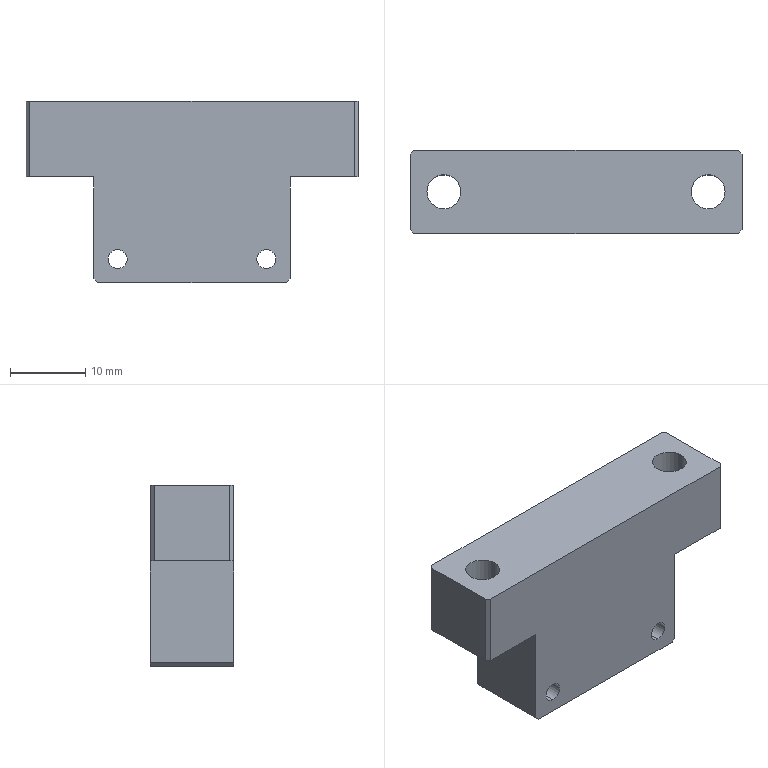Part | SolidWorks | features Chamfer 2, HoleWzd 2, Extrusion 1, ICE 1 | 1 solid | 30 faces | box 44 x 11 x 24 mm | volume 8094 mm3 | plane 18 | cylinder 12 | commonest cylinder face diameters 2.5 x4 4.5 x4 8 x4
STEP:
#1=CARTESIAN_POINT('',(9.85,-5.5,1.85));
#2=VERTEX_POINT('',#1);
#3=CARTESIAN_POINT('',(9.85,-5.5,4.35));
#4=VERTEX_POINT('',#3);
#5=CARTESIAN_POINT('',(9.85,-5.5,3.1));
#6=DIRECTION('',(0.,1.,0.));
#7=DIRECTION('',(0.,0.,1.));
#8=AXIS2_PLACEMENT_3D('',#5,#6,#7);
#9=CIRCLE('',#8,1.25);
#10=EDGE_CURVE('',#2,#4,#9,.T.);
#11=ORIENTED_EDGE('',*,*,#10,.F.);
#12=CARTESIAN_POINT('',(9.85,5.5,1.85));
#13=VERTEX_POINT('',#12);
#14=CARTESIAN_POINT('',(9.85,5.5,1.85));
#15=DIRECTION('',(0.,1.,0.));
#16=VECTOR('',#15,1000.);
#17=LINE('',#14,#16);
#18=EDGE_CURVE('',#2,#13,#17,.T.);
#19=ORIENTED_EDGE('',*,*,#18,.T.);
#20=CARTESIAN_POINT('',(9.85,5.5,4.35));
#21=VERTEX_POINT('',#20);
#22=CARTESIAN_POINT('',(9.85,5.5,3.1));
#23=DIRECTION('',(0.,1.,0.));
#24=DIRECTION('',(0.,0.,1.));
#25=AXIS2_PLACEMENT_3D('',#22,#23,#24);
#26=CIRCLE('',#25,1.25);
#27=EDGE_CURVE('',#13,#21,#26,.T.);
#28=ORIENTED_EDGE('',*,*,#27,.T.);
#29=CARTESIAN_POINT('',(9.85,5.5,4.35));
#30=DIRECTION('',(0.,1.,0.));
#31=VECTOR('',#30,1000.);
#32=LINE('',#29,#31);
#33=EDGE_CURVE('',#4,#21,#32,.T.);
#34=ORIENTED_EDGE('',*,*,#33,.F.);
#35=EDGE_LOOP('',(#11,#19,#28,#34));
#36=FACE_OUTER_BOUND('',#35,.T.);
#37=CARTESIAN_POINT('',(9.85,5.5,3.1));
#38=DIRECTION('',(0.,1.,0.));
#39=DIRECTION('',(0.,0.,1.));
#40=AXIS2_PLACEMENT_3D('',#37,#38,#39);
#41=CYLINDRICAL_SURFACE('',#40,1.25);
#42=ADVANCED_FACE('',(#36),#41,.F.);
#43=CARTESIAN_POINT('',(-9.85,-5.5,1.85));
#44=VERTEX_POINT('',#43);
#45=CARTESIAN_POINT('',(-9.85,-5.5,4.35));
#46=VERTEX_POINT('',#45);
#47=CARTESIAN_POINT('',(-9.85,-5.5,3.1));
#48=DIRECTION('',(0.,1.,0.));
#49=DIRECTION('',(0.,0.,1.));
#50=AXIS2_PLACEMENT_3D('',#47,#48,#49);
#51=CIRCLE('',#50,1.25);
#52=EDGE_CURVE('',#44,#46,#51,.T.);
#53=ORIENTED_EDGE('',*,*,#52,.F.);
#54=CARTESIAN_POINT('',(-9.85,5.5,1.85));
#55=VERTEX_POINT('',#54);
#56=CARTESIAN_POINT('',(-9.85,5.5,1.85));
#57=DIRECTION('',(0.,1.,0.));
#58=VECTOR('',#57,1000.);
#59=LINE('',#56,#58);
#60=EDGE_CURVE('',#44,#55,#59,.T.);
#61=ORIENTED_EDGE('',*,*,#60,.T.);
#62=CARTESIAN_POINT('',(-9.85,5.5,4.35));
#63=VERTEX_POINT('',#62);
#64=CARTESIAN_POINT('',(-9.85,5.5,3.1));
#65=DIRECTION('',(0.,1.,0.));
#66=DIRECTION('',(0.,0.,1.));
#67=AXIS2_PLACEMENT_3D('',#64,#65,#66);
#68=CIRCLE('',#67,1.25);
#69=EDGE_CURVE('',#55,#63,#68,.T.);
#70=ORIENTED_EDGE('',*,*,#69,.T.);
#71=CARTESIAN_POINT('',(-9.85,5.5,4.35));
#72=DIRECTION('',(0.,1.,0.));
#73=VECTOR('',#72,1000.);
#74=LINE('',#71,#73);
#75=EDGE_CURVE('',#46,#63,#74,.T.);
#76=ORIENTED_EDGE('',*,*,#75,.F.);
#77=EDGE_LOOP('',(#53,#61,#70,#76));
#78=FACE_OUTER_BOUND('',#77,.T.);
#79=CARTESIAN_POINT('',(-9.85,5.5,3.1));
#80=DIRECTION('',(0.,1.,0.));
#81=DIRECTION('',(0.,0.,1.));
#82=AXIS2_PLACEMENT_3D('',#79,#80,#81);
#83=CYLINDRICAL_SURFACE('',#82,1.25);
#84=ADVANCED_FACE('',(#78),#83,.F.);
#85=CARTESIAN_POINT('',(21.5,0.,18.6));
#86=VERTEX_POINT('',#85);
#87=CARTESIAN_POINT('',(13.5,0.,18.6));
#88=VERTEX_POINT('',#87);
#89=CARTESIAN_POINT('',(17.5,0.,18.6));
#90=DIRECTION('',(0.,0.,-1.));
#91=DIRECTION('',(-1.,0.,0.));
#92=AXIS2_PLACEMENT_3D('',#89,#90,#91);
#93=CIRCLE('',#92,4.);
#94=EDGE_CURVE('',#86,#88,#93,.T.);
#95=ORIENTED_EDGE('',*,*,#94,.F.);
#96=CARTESIAN_POINT('',(21.5,0.,14.));
#97=VERTEX_POINT('',#96);
#98=CARTESIAN_POINT('',(21.5,0.,14.));
#99=DIRECTION('',(0.,0.,-1.));
#100=VECTOR('',#99,1000.);
#101=LINE('',#98,#100);
#102=EDGE_CURVE('',#86,#97,#101,.T.);
#103=ORIENTED_EDGE('',*,*,#102,.T.);
#104=CARTESIAN_POINT('',(13.5,0.,14.));
#105=VERTEX_POINT('',#104);
#106=CARTESIAN_POINT('',(17.5,0.,14.));
#107=DIRECTION('',(0.,0.,-1.));
#108=DIRECTION('',(-1.,0.,0.));
#109=AXIS2_PLACEMENT_3D('',#106,#107,#108);
#110=CIRCLE('',#109,4.);
#111=EDGE_CURVE('',#97,#105,#110,.T.);
#112=ORIENTED_EDGE('',*,*,#111,.T.);
#113=CARTESIAN_POINT('',(13.5,0.,14.));
#114=DIRECTION('',(0.,0.,-1.));
#115=VECTOR('',#114,1000.);
#116=LINE('',#113,#115);
#117=EDGE_CURVE('',#88,#105,#116,.T.);
#118=ORIENTED_EDGE('',*,*,#117,.F.);
#119=EDGE_LOOP('',(#95,#103,#112,#118));
#120=FACE_OUTER_BOUND('',#119,.T.);
#121=CARTESIAN_POINT('',(17.5,0.,14.));
#122=DIRECTION('',(0.,0.,-1.));
#123=DIRECTION('',(-1.,0.,0.));
#124=AXIS2_PLACEMENT_3D('',#121,#122,#123);
#125=CYLINDRICAL_SURFACE('',#124,4.);
#126=ADVANCED_FACE('',(#120),#125,.F.);
#127=CARTESIAN_POINT('',(19.75,0.,24.));
#128=VERTEX_POINT('',#127);
#129=CARTESIAN_POINT('',(15.25,0.,24.));
#130=VERTEX_POINT('',#129);
#131=CARTESIAN_POINT('',(17.5,0.,24.));
#132=DIRECTION('',(0.,0.,-1.));
#133=DIRECTION('',(-1.,0.,0.));
#134=AXIS2_PLACEMENT_3D('',#131,#132,#133);
#135=CIRCLE('',#134,2.25);
#136=EDGE_CURVE('',#128,#130,#135,.T.);
#137=ORIENTED_EDGE('',*,*,#136,.F.);
#138=CARTESIAN_POINT('',(19.75,0.,18.6));
#139=VERTEX_POINT('',#138);
#140=CARTESIAN_POINT('',(19.75,0.,14.));
#141=DIRECTION('',(0.,0.,-1.));
#142=VECTOR('',#141,1000.);
#143=LINE('',#140,#142);
#144=EDGE_CURVE('',#128,#139,#143,.T.);
#145=ORIENTED_EDGE('',*,*,#144,.T.);
#146=CARTESIAN_POINT('',(15.25,0.,18.6));
#147=VERTEX_POINT('',#146);
#148=CARTESIAN_POINT('',(17.5,0.,18.6));
#149=DIRECTION('',(0.,0.,-1.));
#150=DIRECTION('',(-1.,0.,0.));
#151=AXIS2_PLACEMENT_3D('',#148,#149,#150);
#152=CIRCLE('',#151,2.25);
#153=EDGE_CURVE('',#139,#147,#152,.T.);
#154=ORIENTED_EDGE('',*,*,#153,.T.);
#155=CARTESIAN_POINT('',(15.25,0.,14.));
#156=DIRECTION('',(0.,0.,-1.));
#157=VECTOR('',#156,1000.);
#158=LINE('',#155,#157);
#159=EDGE_CURVE('',#130,#147,#158,.T.);
#160=ORIENTED_EDGE('',*,*,#159,.F.);
#161=EDGE_LOOP('',(#137,#145,#154,#160));
#162=FACE_OUTER_BOUND('',#161,.T.);
#163=CARTESIAN_POINT('',(17.5,0.,14.));
#164=DIRECTION('',(0.,0.,-1.));
#165=DIRECTION('',(-1.,0.,0.));
#166=AXIS2_PLACEMENT_3D('',#163,#164,#165);
#167=CYLINDRICAL_SURFACE('',#166,2.25);
#168=ADVANCED_FACE('',(#162),#167,.F.);
#169=CARTESIAN_POINT('',(-13.5,0.,18.6));
#170=VERTEX_POINT('',#169);
#171=CARTESIAN_POINT('',(-21.5,0.,18.6));
#172=VERTEX_POINT('',#171);
#173=CARTESIAN_POINT('',(-17.5,0.,18.6));
#174=DIRECTION('',(0.,0.,-1.));
#175=DIRECTION('',(-1.,0.,0.));
#176=AXIS2_PLACEMENT_3D('',#173,#174,#175);
#177=CIRCLE('',#176,4.);
#178=EDGE_CURVE('',#170,#172,#177,.T.);
#179=ORIENTED_EDGE('',*,*,#178,.F.);
#180=CARTESIAN_POINT('',(-13.5,0.,14.));
#181=VERTEX_POINT('',#180);
#182=CARTESIAN_POINT('',(-13.5,0.,14.));
#183=DIRECTION('',(0.,0.,-1.));
#184=VECTOR('',#183,1000.);
#185=LINE('',#182,#184);
#186=EDGE_CURVE('',#170,#181,#185,.T.);
#187=ORIENTED_EDGE('',*,*,#186,.T.);
#188=CARTESIAN_POINT('',(-21.5,0.,14.));
#189=VERTEX_POINT('',#188);
#190=CARTESIAN_POINT('',(-17.5,0.,14.));
#191=DIRECTION('',(0.,0.,-1.));
#192=DIRECTION('',(-1.,0.,0.));
#193=AXIS2_PLACEMENT_3D('',#190,#191,#192);
#194=CIRCLE('',#193,4.);
#195=EDGE_CURVE('',#181,#189,#194,.T.);
#196=ORIENTED_EDGE('',*,*,#195,.T.);
#197=CARTESIAN_POINT('',(-21.5,0.,14.));
#198=DIRECTION('',(0.,0.,-1.));
#199=VECTOR('',#198,1000.);
#200=LINE('',#197,#199);
#201=EDGE_CURVE('',#172,#189,#200,.T.);
#202=ORIENTED_EDGE('',*,*,#201,.F.);
#203=EDGE_LOOP('',(#179,#187,#196,#202));
#204=FACE_OUTER_BOUND('',#203,.T.);
#205=CARTESIAN_POINT('',(-17.5,0.,14.));
#206=DIRECTION('',(0.,0.,-1.));
#207=DIRECTION('',(-1.,0.,0.));
#208=AXIS2_PLACEMENT_3D('',#205,#206,#207);
#209=CYLINDRICAL_SURFACE('',#208,4.);
#210=ADVANCED_FACE('',(#204),#209,.F.);
#211=CARTESIAN_POINT('',(-15.25,0.,24.));
#212=VERTEX_POINT('',#211);
#213=CARTESIAN_POINT('',(-19.75,0.,24.));
#214=VERTEX_POINT('',#213);
#215=CARTESIAN_POINT('',(-17.5,0.,24.));
#216=DIRECTION('',(0.,0.,-1.));
#217=DIRECTION('',(-1.,0.,0.));
#218=AXIS2_PLACEMENT_3D('',#215,#216,#217);
#219=CIRCLE('',#218,2.25);
#220=EDGE_CURVE('',#212,#214,#219,.T.);
#221=ORIENTED_EDGE('',*,*,#220,.F.);
#222=CARTESIAN_POINT('',(-15.25,0.,18.6));
#223=VERTEX_POINT('',#222);
#224=CARTESIAN_POINT('',(-15.25,0.,14.));
#225=DIRECTION('',(0.,0.,-1.));
#226=VECTOR('',#225,1000.);
#227=LINE('',#224,#226);
#228=EDGE_CURVE('',#212,#223,#227,.T.);
#229=ORIENTED_EDGE('',*,*,#228,.T.);
#230=CARTESIAN_POINT('',(-19.75,0.,18.6));
#231=VERTEX_POINT('',#230);
#232=CARTESIAN_POINT('',(-17.5,0.,18.6));
#233=DIRECTION('',(0.,0.,-1.));
#234=DIRECTION('',(-1.,0.,0.));
#235=AXIS2_PLACEMENT_3D('',#232,#233,#234);
#236=CIRCLE('',#235,2.25);
#237=EDGE_CURVE('',#223,#231,#236,.T.);
#238=ORIENTED_EDGE('',*,*,#237,.T.);
#239=CARTESIAN_POINT('',(-19.75,0.,14.));
#240=DIRECTION('',(0.,0.,-1.));
#241=VECTOR('',#240,1000.);
#242=LINE('',#239,#241);
#243=EDGE_CURVE('',#214,#231,#242,.T.);
#244=ORIENTED_EDGE('',*,*,#243,.F.);
#245=EDGE_LOOP('',(#221,#229,#238,#244));
#246=FACE_OUTER_BOUND('',#245,.T.);
#247=CARTESIAN_POINT('',(-17.5,0.,14.));
#248=DIRECTION('',(0.,0.,-1.));
#249=DIRECTION('',(-1.,0.,0.));
#250=AXIS2_PLACEMENT_3D('',#247,#248,#249);
#251=CYLINDRICAL_SURFACE('',#250,2.25);
#252=ADVANCED_FACE('',(#246),#251,.F.);
#253=CARTESIAN_POINT('',(13.,5.5,14.));
#254=VERTEX_POINT('',#253);
#255=CARTESIAN_POINT('',(21.5,5.5,14.));
#256=VERTEX_POINT('',#255);
#257=CARTESIAN_POINT('',(22.,5.5,14.));
#258=DIRECTION('',(1.,0.,0.));
#259=VECTOR('',#258,1000.);
#260=LINE('',#257,#259);
#261=EDGE_CURVE('',#254,#256,#260,.T.);
#262=ORIENTED_EDGE('',*,*,#261,.T.);
#263=CARTESIAN_POINT('',(22.,5.,14.));
#264=VERTEX_POINT('',#263);
#265=CARTESIAN_POINT('',(21.5,5.5,14.));
#266=DIRECTION('',(0.7071,-0.7071,0.));
#267=VECTOR('',#266,1000.);
#268=LINE('',#265,#267);
#269=EDGE_CURVE('',#256,#264,#268,.T.);
#270=ORIENTED_EDGE('',*,*,#269,.T.);
#271=CARTESIAN_POINT('',(22.,-5.,14.));
#272=VERTEX_POINT('',#271);
#273=CARTESIAN_POINT('',(22.,-5.5,14.));
#274=DIRECTION('',(0.,1.,0.));
#275=VECTOR('',#274,1000.);
#276=LINE('',#273,#275);
#277=EDGE_CURVE('',#272,#264,#276,.T.);
#278=ORIENTED_EDGE('',*,*,#277,.F.);
#279=CARTESIAN_POINT('',(21.5,-5.5,14.));
#280=VERTEX_POINT('',#279);
#281=CARTESIAN_POINT('',(22.,-5.,14.));
#282=DIRECTION('',(-0.7071,-0.7071,0.));
#283=VECTOR('',#282,1000.);
#284=LINE('',#281,#283);
#285=EDGE_CURVE('',#272,#280,#284,.T.);
#286=ORIENTED_EDGE('',*,*,#285,.T.);
#287=CARTESIAN_POINT('',(13.,-5.5,14.));
#288=VERTEX_POINT('',#287);
#289=CARTESIAN_POINT('',(22.,-5.5,14.));
#290=DIRECTION('',(1.,0.,0.));
#291=VECTOR('',#290,1000.);
#292=LINE('',#289,#291);
#293=EDGE_CURVE('',#288,#280,#292,.T.);
#294=ORIENTED_EDGE('',*,*,#293,.F.);
#295=CARTESIAN_POINT('',(13.,-5.5,14.));
#296=DIRECTION('',(0.,1.,0.));
#297=VECTOR('',#296,1000.);
#298=LINE('',#295,#297);
#299=EDGE_CURVE('',#288,#254,#298,.T.);
#300=ORIENTED_EDGE('',*,*,#299,.T.);
#301=EDGE_LOOP('',(#262,#270,#278,#286,#294,#300));
#302=FACE_OUTER_BOUND('',#301,.T.);
#303=CARTESIAN_POINT('',(17.5,0.,14.));
#304=DIRECTION('',(0.,0.,-1.));
#305=DIRECTION('',(-1.,0.,0.));
#306=AXIS2_PLACEMENT_3D('',#303,#304,#305);
#307=CIRCLE('',#306,4.);
#308=EDGE_CURVE('',#105,#97,#307,.T.);
#309=ORIENTED_EDGE('',*,*,#308,.F.);
#310=ORIENTED_EDGE('',*,*,#111,.F.);
#311=EDGE_LOOP('',(#309,#310));
#312=FACE_BOUND('',#311,.T.);
#313=CARTESIAN_POINT('',(22.,-5.5,14.));
#314=DIRECTION('',(0.,0.,1.));
#315=DIRECTION('',(1.,0.,0.));
#316=AXIS2_PLACEMENT_3D('',#313,#314,#315);
#317=PLANE('',#316);
#318=ADVANCED_FACE('',(#302,#312),#317,.F.);
#319=ORIENTED_EDGE('',*,*,#277,.T.);
#320=CARTESIAN_POINT('',(22.,5.,24.));
#321=VERTEX_POINT('',#320);
#322=CARTESIAN_POINT('',(22.,5.,24.));
#323=DIRECTION('',(0.,0.,1.));
#324=VECTOR('',#323,1000.);
#325=LINE('',#322,#324);
#326=EDGE_CURVE('',#264,#321,#325,.T.);
#327=ORIENTED_EDGE('',*,*,#326,.T.);
#328=CARTESIAN_POINT('',(22.,-5.,24.));
#329=VERTEX_POINT('',#328);
#330=CARTESIAN_POINT('',(22.,5.5,24.));
#331=DIRECTION('',(0.,1.,0.));
#332=VECTOR('',#331,1000.);
#333=LINE('',#330,#332);
#334=EDGE_CURVE('',#329,#321,#333,.T.);
#335=ORIENTED_EDGE('',*,*,#334,.F.);
#336=CARTESIAN_POINT('',(22.,-5.,24.));
#337=DIRECTION('',(0.,0.,-1.));
#338=VECTOR('',#337,1000.);
#339=LINE('',#336,#338);
#340=EDGE_CURVE('',#329,#272,#339,.T.);
#341=ORIENTED_EDGE('',*,*,#340,.T.);
#342=EDGE_LOOP('',(#319,#327,#335,#341));
#343=FACE_OUTER_BOUND('',#342,.T.);
#344=CARTESIAN_POINT('',(22.,5.5,24.));
#345=DIRECTION('',(-1.,0.,0.));
#346=DIRECTION('',(0.,0.,1.));
#347=AXIS2_PLACEMENT_3D('',#344,#345,#346);
#348=PLANE('',#347);
#349=ADVANCED_FACE('',(#343),#348,.F.);
#350=CARTESIAN_POINT('',(9.85,5.5,3.1));
#351=DIRECTION('',(0.,1.,0.));
#352=DIRECTION('',(0.,0.,1.));
#353=AXIS2_PLACEMENT_3D('',#350,#351,#352);
#354=CIRCLE('',#353,1.25);
#355=EDGE_CURVE('',#21,#13,#354,.T.);
#356=ORIENTED_EDGE('',*,*,#355,.F.);
#357=ORIENTED_EDGE('',*,*,#27,.F.);
#358=EDGE_LOOP('',(#356,#357));
#359=FACE_BOUND('',#358,.T.);
#360=CARTESIAN_POINT('',(-9.85,5.5,3.1));
#361=DIRECTION('',(0.,1.,0.));
#362=DIRECTION('',(0.,0.,1.));
#363=AXIS2_PLACEMENT_3D('',#360,#361,#362);
#364=CIRCLE('',#363,1.25);
#365=EDGE_CURVE('',#63,#55,#364,.T.);
#366=ORIENTED_EDGE('',*,*,#365,.F.);
#367=ORIENTED_EDGE('',*,*,#69,.F.);
#368=EDGE_LOOP('',(#366,#367));
#369=FACE_BOUND('',#368,.T.);
#370=CARTESIAN_POINT('',(13.,5.5,0.5));
#371=VERTEX_POINT('',#370);
#372=CARTESIAN_POINT('',(13.,5.5,14.));
#373=DIRECTION('',(0.,0.,1.));
#374=VECTOR('',#373,1000.);
#375=LINE('',#372,#374);
#376=EDGE_CURVE('',#371,#254,#375,.T.);
#377=ORIENTED_EDGE('',*,*,#376,.F.);
#378=CARTESIAN_POINT('',(12.5,5.5,0.));
#379=VERTEX_POINT('',#378);
#380=CARTESIAN_POINT('',(13.,5.5,0.5));
#381=DIRECTION('',(-0.7071,0.,-0.7071));
#382=VECTOR('',#381,1000.);
#383=LINE('',#380,#382);
#384=EDGE_CURVE('',#371,#379,#383,.T.);
#385=ORIENTED_EDGE('',*,*,#384,.T.);
#386=CARTESIAN_POINT('',(-12.5,5.5,0.));
#387=VERTEX_POINT('',#386);
#388=CARTESIAN_POINT('',(-22.,5.5,0.));
#389=DIRECTION('',(-1.,0.,0.));
#390=VECTOR('',#389,1000.);
#391=LINE('',#388,#390);
#392=EDGE_CURVE('',#379,#387,#391,.T.);
#393=ORIENTED_EDGE('',*,*,#392,.T.);
#394=CARTESIAN_POINT('',(-13.,5.5,0.5));
#395=VERTEX_POINT('',#394);
#396=CARTESIAN_POINT('',(-12.5,5.5,0.));
#397=DIRECTION('',(-0.7071,0.,0.7071));
#398=VECTOR('',#397,1000.);
#399=LINE('',#396,#398);
#400=EDGE_CURVE('',#387,#395,#399,.T.);
#401=ORIENTED_EDGE('',*,*,#400,.T.);
#402=CARTESIAN_POINT('',(-13.,5.5,14.));
#403=VERTEX_POINT('',#402);
#404=CARTESIAN_POINT('',(-13.,5.5,14.));
#405=DIRECTION('',(0.,0.,-1.));
#406=VECTOR('',#405,1000.);
#407=LINE('',#404,#406);
#408=EDGE_CURVE('',#403,#395,#407,.T.);
#409=ORIENTED_EDGE('',*,*,#408,.F.);
#410=CARTESIAN_POINT('',(-21.5,5.5,14.));
#411=VERTEX_POINT('',#410);
#412=CARTESIAN_POINT('',(-22.,5.5,14.));
#413=DIRECTION('',(1.,0.,0.));
#414=VECTOR('',#413,1000.);
#415=LINE('',#412,#414);
#416=EDGE_CURVE('',#411,#403,#415,.T.);
#417=ORIENTED_EDGE('',*,*,#416,.F.);
#418=CARTESIAN_POINT('',(-21.5,5.5,24.));
#419=VERTEX_POINT('',#418);
#420=CARTESIAN_POINT('',(-21.5,5.5,24.));
#421=DIRECTION('',(0.,0.,1.));
#422=VECTOR('',#421,1000.);
#423=LINE('',#420,#422);
#424=EDGE_CURVE('',#411,#419,#423,.T.);
#425=ORIENTED_EDGE('',*,*,#424,.T.);
#426=CARTESIAN_POINT('',(21.5,5.5,24.));
#427=VERTEX_POINT('',#426);
#428=CARTESIAN_POINT('',(-22.,5.5,24.));
#429=DIRECTION('',(-1.,0.,0.));
#430=VECTOR('',#429,1000.);
#431=LINE('',#428,#430);
#432=EDGE_CURVE('',#427,#419,#431,.T.);
#433=ORIENTED_EDGE('',*,*,#432,.F.);
#434=CARTESIAN_POINT('',(21.5,5.5,24.));
#435=DIRECTION('',(0.,0.,-1.));
#436=VECTOR('',#435,1000.);
#437=LINE('',#434,#436);
#438=EDGE_CURVE('',#427,#256,#437,.T.);
#439=ORIENTED_EDGE('',*,*,#438,.T.);
#440=ORIENTED_EDGE('',*,*,#261,.F.);
#441=EDGE_LOOP('',(#377,#385,#393,#401,#409,#417,#425,#433,#439,#440));
#442=FACE_OUTER_BOUND('',#441,.T.);
#443=CARTESIAN_POINT('',(-22.,5.5,24.));
#444=DIRECTION('',(0.,-1.,0.));
#445=DIRECTION('',(0.,0.,-1.));
#446=AXIS2_PLACEMENT_3D('',#443,#444,#445);
#447=PLANE('',#446);
#448=ADVANCED_FACE('',(#359,#369,#442),#447,.F.);
#449=CARTESIAN_POINT('',(-22.,5.,24.));
#450=VERTEX_POINT('',#449);
#451=CARTESIAN_POINT('',(-22.,-5.,24.));
#452=VERTEX_POINT('',#451);
#453=CARTESIAN_POINT('',(-22.,5.5,24.));
#454=DIRECTION('',(0.,-1.,0.));
#455=VECTOR('',#454,1000.);
#456=LINE('',#453,#455);
#457=EDGE_CURVE('',#450,#452,#456,.T.);
#458=ORIENTED_EDGE('',*,*,#457,.F.);
#459=CARTESIAN_POINT('',(-22.,5.,14.));
#460=VERTEX_POINT('',#459);
#461=CARTESIAN_POINT('',(-22.,5.,24.));
#462=DIRECTION('',(0.,0.,-1.));
#463=VECTOR('',#462,1000.);
#464=LINE('',#461,#463);
#465=EDGE_CURVE('',#450,#460,#464,.T.);
#466=ORIENTED_EDGE('',*,*,#465,.T.);
#467=CARTESIAN_POINT('',(-22.,-5.,14.));
#468=VERTEX_POINT('',#467);
#469=CARTESIAN_POINT('',(-22.,-5.5,14.));
#470=DIRECTION('',(0.,1.,0.));
#471=VECTOR('',#470,1000.);
#472=LINE('',#469,#471);
#473=EDGE_CURVE('',#468,#460,#472,.T.);
#474=ORIENTED_EDGE('',*,*,#473,.F.);
#475=CARTESIAN_POINT('',(-22.,-5.,24.));
#476=DIRECTION('',(0.,0.,1.));
#477=VECTOR('',#476,1000.);
#478=LINE('',#475,#477);
#479=EDGE_CURVE('',#468,#452,#478,.T.);
#480=ORIENTED_EDGE('',*,*,#479,.T.);
#481=EDGE_LOOP('',(#458,#466,#474,#480));
#482=FACE_OUTER_BOUND('',#481,.T.);
#483=CARTESIAN_POINT('',(-22.,5.5,24.));
#484=DIRECTION('',(1.,0.,0.));
#485=DIRECTION('',(0.,0.,-1.));
#486=AXIS2_PLACEMENT_3D('',#483,#484,#485);
#487=PLANE('',#486);
#488=ADVANCED_FACE('',(#482),#487,.F.);
#489=CARTESIAN_POINT('',(9.85,-5.5,3.1));
#490=DIRECTION('',(0.,1.,0.));
#491=DIRECTION('',(0.,0.,1.));
#492=AXIS2_PLACEMENT_3D('',#489,#490,#491);
#493=CIRCLE('',#492,1.25);
#494=EDGE_CURVE('',#4,#2,#493,.T.);
#495=ORIENTED_EDGE('',*,*,#494,.T.);
#496=ORIENTED_EDGE('',*,*,#10,.T.);
#497=EDGE_LOOP('',(#495,#496));
#498=FACE_BOUND('',#497,.T.);
#499=CARTESIAN_POINT('',(-9.85,-5.5,3.1));
#500=DIRECTION('',(0.,1.,0.));
#501=DIRECTION('',(0.,0.,1.));
#502=AXIS2_PLACEMENT_3D('',#499,#500,#501);
#503=CIRCLE('',#502,1.25);
#504=EDGE_CURVE('',#46,#44,#503,.T.);
#505=ORIENTED_EDGE('',*,*,#504,.T.);
#506=ORIENTED_EDGE('',*,*,#52,.T.);
#507=EDGE_LOOP('',(#505,#506));
#508=FACE_BOUND('',#507,.T.);
#509=CARTESIAN_POINT('',(-12.5,-5.5,0.));
#510=VERTEX_POINT('',#509);
#511=CARTESIAN_POINT('',(12.5,-5.5,0.));
#512=VERTEX_POINT('',#511);
#513=CARTESIAN_POINT('',(-22.,-5.5,0.));
#514=DIRECTION('',(1.,0.,0.));
#515=VECTOR('',#514,1000.);
#516=LINE('',#513,#515);
#517=EDGE_CURVE('',#510,#512,#516,.T.);
#518=ORIENTED_EDGE('',*,*,#517,.T.);
#519=CARTESIAN_POINT('',(13.,-5.5,0.5));
#520=VERTEX_POINT('',#519);
#521=CARTESIAN_POINT('',(13.,-5.5,0.5));
#522=DIRECTION('',(0.7071,0.,0.7071));
#523=VECTOR('',#522,1000.);
#524=LINE('',#521,#523);
#525=EDGE_CURVE('',#512,#520,#524,.T.);
#526=ORIENTED_EDGE('',*,*,#525,.T.);
#527=CARTESIAN_POINT('',(13.,-5.5,14.));
#528=DIRECTION('',(0.,0.,1.));
#529=VECTOR('',#528,1000.);
#530=LINE('',#527,#529);
#531=EDGE_CURVE('',#520,#288,#530,.T.);
#532=ORIENTED_EDGE('',*,*,#531,.T.);
#533=ORIENTED_EDGE('',*,*,#293,.T.);
#534=CARTESIAN_POINT('',(21.5,-5.5,24.));
#535=VERTEX_POINT('',#534);
#536=CARTESIAN_POINT('',(21.5,-5.5,24.));
#537=DIRECTION('',(0.,0.,1.));
#538=VECTOR('',#537,1000.);
#539=LINE('',#536,#538);
#540=EDGE_CURVE('',#280,#535,#539,.T.);
#541=ORIENTED_EDGE('',*,*,#540,.T.);
#542=CARTESIAN_POINT('',(-21.5,-5.5,24.));
#543=VERTEX_POINT('',#542);
#544=CARTESIAN_POINT('',(-22.,-5.5,24.));
#545=DIRECTION('',(1.,0.,0.));
#546=VECTOR('',#545,1000.);
#547=LINE('',#544,#546);
#548=EDGE_CURVE('',#543,#535,#547,.T.);
#549=ORIENTED_EDGE('',*,*,#548,.F.);
#550=CARTESIAN_POINT('',(-21.5,-5.5,14.));
#551=VERTEX_POINT('',#550);
#552=CARTESIAN_POINT('',(-21.5,-5.5,24.));
#553=DIRECTION('',(0.,0.,-1.));
#554=VECTOR('',#553,1000.);
#555=LINE('',#552,#554);
#556=EDGE_CURVE('',#543,#551,#555,.T.);
#557=ORIENTED_EDGE('',*,*,#556,.T.);
#558=CARTESIAN_POINT('',(-13.,-5.5,14.));
#559=VERTEX_POINT('',#558);
#560=CARTESIAN_POINT('',(-22.,-5.5,14.));
#561=DIRECTION('',(1.,0.,0.));
#562=VECTOR('',#561,1000.);
#563=LINE('',#560,#562);
#564=EDGE_CURVE('',#551,#559,#563,.T.);
#565=ORIENTED_EDGE('',*,*,#564,.T.);
#566=CARTESIAN_POINT('',(-13.,-5.5,0.5));
#567=VERTEX_POINT('',#566);
#568=CARTESIAN_POINT('',(-13.,-5.5,14.));
#569=DIRECTION('',(0.,0.,-1.));
#570=VECTOR('',#569,1000.);
#571=LINE('',#568,#570);
#572=EDGE_CURVE('',#559,#567,#571,.T.);
#573=ORIENTED_EDGE('',*,*,#572,.T.);
#574=CARTESIAN_POINT('',(-12.5,-5.5,0.));
#575=DIRECTION('',(0.7071,0.,-0.7071));
#576=VECTOR('',#575,1000.);
#577=LINE('',#574,#576);
#578=EDGE_CURVE('',#567,#510,#577,.T.);
#579=ORIENTED_EDGE('',*,*,#578,.T.);
#580=EDGE_LOOP('',(#518,#526,#532,#533,#541,#549,#557,#565,#573,#579));
#581=FACE_OUTER_BOUND('',#580,.T.);
#582=CARTESIAN_POINT('',(-22.,-5.5,24.));
#583=DIRECTION('',(0.,1.,0.));
#584=DIRECTION('',(0.,0.,1.));
#585=AXIS2_PLACEMENT_3D('',#582,#583,#584);
#586=PLANE('',#585);
#587=ADVANCED_FACE('',(#498,#508,#581),#586,.F.);
#588=CARTESIAN_POINT('',(17.5,0.,24.));
#589=DIRECTION('',(0.,0.,-1.));
#590=DIRECTION('',(-1.,0.,0.));
#591=AXIS2_PLACEMENT_3D('',#588,#589,#590);
#592=CIRCLE('',#591,2.25);
#593=EDGE_CURVE('',#130,#128,#592,.T.);
#594=ORIENTED_EDGE('',*,*,#593,.T.);
#595=ORIENTED_EDGE('',*,*,#136,.T.);
#596=EDGE_LOOP('',(#594,#595));
#597=FACE_BOUND('',#596,.T.);
#598=CARTESIAN_POINT('',(-17.5,0.,24.));
#599=DIRECTION('',(0.,0.,-1.));
#600=DIRECTION('',(-1.,0.,0.));
#601=AXIS2_PLACEMENT_3D('',#598,#599,#600);
#602=CIRCLE('',#601,2.25);
#603=EDGE_CURVE('',#214,#212,#602,.T.);
#604=ORIENTED_EDGE('',*,*,#603,.T.);
#605=ORIENTED_EDGE('',*,*,#220,.T.);
#606=EDGE_LOOP('',(#604,#605));
#607=FACE_BOUND('',#606,.T.);
#608=ORIENTED_EDGE('',*,*,#334,.T.);
#609=CARTESIAN_POINT('',(13.5,13.5,24.));
#610=DIRECTION('',(-0.7071,0.7071,0.));
#611=VECTOR('',#610,1000.);
#612=LINE('',#609,#611);
#613=EDGE_CURVE('',#321,#427,#612,.T.);
#614=ORIENTED_EDGE('',*,*,#613,.T.);
#615=ORIENTED_EDGE('',*,*,#432,.T.);
#616=CARTESIAN_POINT('',(-13.5,13.5,24.));
#617=DIRECTION('',(-0.7071,-0.7071,0.));
#618=VECTOR('',#617,1000.);
#619=LINE('',#616,#618);
#620=EDGE_CURVE('',#419,#450,#619,.T.);
#621=ORIENTED_EDGE('',*,*,#620,.T.);
#622=ORIENTED_EDGE('',*,*,#457,.T.);
#623=CARTESIAN_POINT('',(-13.5,-13.5,24.));
#624=DIRECTION('',(0.7071,-0.7071,0.));
#625=VECTOR('',#624,1000.);
#626=LINE('',#623,#625);
#627=EDGE_CURVE('',#452,#543,#626,.T.);
#628=ORIENTED_EDGE('',*,*,#627,.T.);
#629=ORIENTED_EDGE('',*,*,#548,.T.);
#630=CARTESIAN_POINT('',(13.5,-13.5,24.));
#631=DIRECTION('',(0.7071,0.7071,0.));
#632=VECTOR('',#631,1000.);
#633=LINE('',#630,#632);
#634=EDGE_CURVE('',#535,#329,#633,.T.);
#635=ORIENTED_EDGE('',*,*,#634,.T.);
#636=EDGE_LOOP('',(#608,#614,#615,#621,#622,#628,#629,#635));
#637=FACE_OUTER_BOUND('',#636,.T.);
#638=CARTESIAN_POINT('',(0.,0.,24.));
#639=DIRECTION('',(0.,0.,1.));
#640=DIRECTION('',(1.,0.,0.));
#641=AXIS2_PLACEMENT_3D('',#638,#639,#640);
#642=PLANE('',#641);
#643=ADVANCED_FACE('',(#597,#607,#637),#642,.T.);
#644=ORIENTED_EDGE('',*,*,#392,.F.);
#645=CARTESIAN_POINT('',(12.5,0.,0.));
#646=DIRECTION('',(0.,-1.,0.));
#647=VECTOR('',#646,1000.);
#648=LINE('',#645,#647);
#649=EDGE_CURVE('',#379,#512,#648,.T.);
#650=ORIENTED_EDGE('',*,*,#649,.T.);
#651=ORIENTED_EDGE('',*,*,#517,.F.);
#652=CARTESIAN_POINT('',(-12.5,0.,0.));
#653=DIRECTION('',(0.,1.,0.));
#654=VECTOR('',#653,1000.);
#655=LINE('',#652,#654);
#656=EDGE_CURVE('',#510,#387,#655,.T.);
#657=ORIENTED_EDGE('',*,*,#656,.T.);
#658=EDGE_LOOP('',(#644,#650,#651,#657));
#659=FACE_OUTER_BOUND('',#658,.T.);
#660=CARTESIAN_POINT('',(0.,0.,0.));
#661=DIRECTION('',(0.,0.,1.));
#662=DIRECTION('',(1.,0.,0.));
#663=AXIS2_PLACEMENT_3D('',#660,#661,#662);
#664=PLANE('',#663);
#665=ADVANCED_FACE('',(#659),#664,.F.);
#666=ORIENTED_EDGE('',*,*,#531,.F.);
#667=CARTESIAN_POINT('',(13.,-5.5,0.5));
#668=DIRECTION('',(0.,1.,0.));
#669=VECTOR('',#668,1000.);
#670=LINE('',#667,#669);
#671=EDGE_CURVE('',#520,#371,#670,.T.);
#672=ORIENTED_EDGE('',*,*,#671,.T.);
#673=ORIENTED_EDGE('',*,*,#376,.T.);
#674=ORIENTED_EDGE('',*,*,#299,.F.);
#675=EDGE_LOOP('',(#666,#672,#673,#674));
#676=FACE_OUTER_BOUND('',#675,.T.);
#677=CARTESIAN_POINT('',(13.,-5.5,14.));
#678=DIRECTION('',(-1.,0.,0.));
#679=DIRECTION('',(0.,0.,1.));
#680=AXIS2_PLACEMENT_3D('',#677,#678,#679);
#681=PLANE('',#680);
#682=ADVANCED_FACE('',(#676),#681,.F.);
#683=ORIENTED_EDGE('',*,*,#408,.T.);
#684=CARTESIAN_POINT('',(-13.,-5.5,0.5));
#685=DIRECTION('',(0.,-1.,0.));
#686=VECTOR('',#685,1000.);
#687=LINE('',#684,#686);
#688=EDGE_CURVE('',#395,#567,#687,.T.);
#689=ORIENTED_EDGE('',*,*,#688,.T.);
#690=ORIENTED_EDGE('',*,*,#572,.F.);
#691=CARTESIAN_POINT('',(-13.,-5.5,14.));
#692=DIRECTION('',(0.,1.,0.));
#693=VECTOR('',#692,1000.);
#694=LINE('',#691,#693);
#695=EDGE_CURVE('',#559,#403,#694,.T.);
#696=ORIENTED_EDGE('',*,*,#695,.T.);
#697=EDGE_LOOP('',(#683,#689,#690,#696));
#698=FACE_OUTER_BOUND('',#697,.T.);
#699=CARTESIAN_POINT('',(-13.,-5.5,14.));
#700=DIRECTION('',(1.,0.,0.));
#701=DIRECTION('',(0.,0.,-1.));
#702=AXIS2_PLACEMENT_3D('',#699,#700,#701);
#703=PLANE('',#702);
#704=ADVANCED_FACE('',(#698),#703,.F.);
#705=CARTESIAN_POINT('',(-17.5,0.,14.));
#706=DIRECTION('',(0.,0.,-1.));
#707=DIRECTION('',(-1.,0.,0.));
#708=AXIS2_PLACEMENT_3D('',#705,#706,#707);
#709=CIRCLE('',#708,4.);
#710=EDGE_CURVE('',#189,#181,#709,.T.);
#711=ORIENTED_EDGE('',*,*,#710,.F.);
#712=ORIENTED_EDGE('',*,*,#195,.F.);
#713=EDGE_LOOP('',(#711,#712));
#714=FACE_BOUND('',#713,.T.);
#715=ORIENTED_EDGE('',*,*,#473,.T.);
#716=CARTESIAN_POINT('',(-22.,5.,14.));
#717=DIRECTION('',(0.7071,0.7071,0.));
#718=VECTOR('',#717,1000.);
#719=LINE('',#716,#718);
#720=EDGE_CURVE('',#460,#411,#719,.T.);
#721=ORIENTED_EDGE('',*,*,#720,.T.);
#722=ORIENTED_EDGE('',*,*,#416,.T.);
#723=ORIENTED_EDGE('',*,*,#695,.F.);
#724=ORIENTED_EDGE('',*,*,#564,.F.);
#725=CARTESIAN_POINT('',(-21.5,-5.5,14.));
#726=DIRECTION('',(-0.7071,0.7071,0.));
#727=VECTOR('',#726,1000.);
#728=LINE('',#725,#727);
#729=EDGE_CURVE('',#551,#468,#728,.T.);
#730=ORIENTED_EDGE('',*,*,#729,.T.);
#731=EDGE_LOOP('',(#715,#721,#722,#723,#724,#730));
#732=FACE_OUTER_BOUND('',#731,.T.);
#733=CARTESIAN_POINT('',(-22.,-5.5,14.));
#734=DIRECTION('',(0.,0.,1.));
#735=DIRECTION('',(1.,0.,0.));
#736=AXIS2_PLACEMENT_3D('',#733,#734,#735);
#737=PLANE('',#736);
#738=ADVANCED_FACE('',(#714,#732),#737,.F.);
#739=ORIENTED_EDGE('',*,*,#228,.F.);
#740=ORIENTED_EDGE('',*,*,#603,.F.);
#741=ORIENTED_EDGE('',*,*,#243,.T.);
#742=CARTESIAN_POINT('',(-17.5,0.,18.6));
#743=DIRECTION('',(0.,0.,-1.));
#744=DIRECTION('',(-1.,0.,0.));
#745=AXIS2_PLACEMENT_3D('',#742,#743,#744);
#746=CIRCLE('',#745,2.25);
#747=EDGE_CURVE('',#231,#223,#746,.T.);
#748=ORIENTED_EDGE('',*,*,#747,.T.);
#749=EDGE_LOOP('',(#739,#740,#741,#748));
#750=FACE_OUTER_BOUND('',#749,.T.);
#751=CARTESIAN_POINT('',(-17.5,0.,14.));
#752=DIRECTION('',(0.,0.,-1.));
#753=DIRECTION('',(-1.,0.,0.));
#754=AXIS2_PLACEMENT_3D('',#751,#752,#753);
#755=CYLINDRICAL_SURFACE('',#754,2.25);
#756=ADVANCED_FACE('',(#750),#755,.F.);
#757=ORIENTED_EDGE('',*,*,#747,.F.);
#758=ORIENTED_EDGE('',*,*,#237,.F.);
#759=EDGE_LOOP('',(#757,#758));
#760=FACE_BOUND('',#759,.T.);
#761=CARTESIAN_POINT('',(-17.5,0.,18.6));
#762=DIRECTION('',(0.,0.,-1.));
#763=DIRECTION('',(-1.,0.,0.));
#764=AXIS2_PLACEMENT_3D('',#761,#762,#763);
#765=CIRCLE('',#764,4.);
#766=EDGE_CURVE('',#172,#170,#765,.T.);
#767=ORIENTED_EDGE('',*,*,#766,.T.);
#768=ORIENTED_EDGE('',*,*,#178,.T.);
#769=EDGE_LOOP('',(#767,#768));
#770=FACE_OUTER_BOUND('',#769,.T.);
#771=CARTESIAN_POINT('',(-15.25,0.,18.6));
#772=DIRECTION('',(0.,0.,1.));
#773=DIRECTION('',(1.,0.,0.));
#774=AXIS2_PLACEMENT_3D('',#771,#772,#773);
#775=PLANE('',#774);
#776=ADVANCED_FACE('',(#760,#770),#775,.F.);
#777=ORIENTED_EDGE('',*,*,#186,.F.);
#778=ORIENTED_EDGE('',*,*,#766,.F.);
#779=ORIENTED_EDGE('',*,*,#201,.T.);
#780=ORIENTED_EDGE('',*,*,#710,.T.);
#781=EDGE_LOOP('',(#777,#778,#779,#780));
#782=FACE_OUTER_BOUND('',#781,.T.);
#783=CARTESIAN_POINT('',(-17.5,0.,14.));
#784=DIRECTION('',(0.,0.,-1.));
#785=DIRECTION('',(-1.,0.,0.));
#786=AXIS2_PLACEMENT_3D('',#783,#784,#785);
#787=CYLINDRICAL_SURFACE('',#786,4.);
#788=ADVANCED_FACE('',(#782),#787,.F.);
#789=ORIENTED_EDGE('',*,*,#144,.F.);
#790=ORIENTED_EDGE('',*,*,#593,.F.);
#791=ORIENTED_EDGE('',*,*,#159,.T.);
#792=CARTESIAN_POINT('',(17.5,0.,18.6));
#793=DIRECTION('',(0.,0.,-1.));
#794=DIRECTION('',(-1.,0.,0.));
#795=AXIS2_PLACEMENT_3D('',#792,#793,#794);
#796=CIRCLE('',#795,2.25);
#797=EDGE_CURVE('',#147,#139,#796,.T.);
#798=ORIENTED_EDGE('',*,*,#797,.T.);
#799=EDGE_LOOP('',(#789,#790,#791,#798));
#800=FACE_OUTER_BOUND('',#799,.T.);
#801=CARTESIAN_POINT('',(17.5,0.,14.));
#802=DIRECTION('',(0.,0.,-1.));
#803=DIRECTION('',(-1.,0.,0.));
#804=AXIS2_PLACEMENT_3D('',#801,#802,#803);
#805=CYLINDRICAL_SURFACE('',#804,2.25);
#806=ADVANCED_FACE('',(#800),#805,.F.);
#807=ORIENTED_EDGE('',*,*,#797,.F.);
#808=ORIENTED_EDGE('',*,*,#153,.F.);
#809=EDGE_LOOP('',(#807,#808));
#810=FACE_BOUND('',#809,.T.);
#811=CARTESIAN_POINT('',(17.5,0.,18.6));
#812=DIRECTION('',(0.,0.,-1.));
#813=DIRECTION('',(-1.,0.,0.));
#814=AXIS2_PLACEMENT_3D('',#811,#812,#813);
#815=CIRCLE('',#814,4.);
#816=EDGE_CURVE('',#88,#86,#815,.T.);
#817=ORIENTED_EDGE('',*,*,#816,.T.);
#818=ORIENTED_EDGE('',*,*,#94,.T.);
#819=EDGE_LOOP('',(#817,#818));
#820=FACE_OUTER_BOUND('',#819,.T.);
#821=CARTESIAN_POINT('',(19.75,0.,18.6));
#822=DIRECTION('',(0.,0.,1.));
#823=DIRECTION('',(1.,0.,0.));
#824=AXIS2_PLACEMENT_3D('',#821,#822,#823);
#825=PLANE('',#824);
#826=ADVANCED_FACE('',(#810,#820),#825,.F.);
#827=ORIENTED_EDGE('',*,*,#102,.F.);
#828=ORIENTED_EDGE('',*,*,#816,.F.);
#829=ORIENTED_EDGE('',*,*,#117,.T.);
#830=ORIENTED_EDGE('',*,*,#308,.T.);
#831=EDGE_LOOP('',(#827,#828,#829,#830));
#832=FACE_OUTER_BOUND('',#831,.T.);
#833=CARTESIAN_POINT('',(17.5,0.,14.));
#834=DIRECTION('',(0.,0.,-1.));
#835=DIRECTION('',(-1.,0.,0.));
#836=AXIS2_PLACEMENT_3D('',#833,#834,#835);
#837=CYLINDRICAL_SURFACE('',#836,4.);
#838=ADVANCED_FACE('',(#832),#837,.F.);
#839=ORIENTED_EDGE('',*,*,#60,.F.);
#840=ORIENTED_EDGE('',*,*,#504,.F.);
#841=ORIENTED_EDGE('',*,*,#75,.T.);
#842=ORIENTED_EDGE('',*,*,#365,.T.);
#843=EDGE_LOOP('',(#839,#840,#841,#842));
#844=FACE_OUTER_BOUND('',#843,.T.);
#845=CARTESIAN_POINT('',(-9.85,5.5,3.1));
#846=DIRECTION('',(0.,1.,0.));
#847=DIRECTION('',(0.,0.,1.));
#848=AXIS2_PLACEMENT_3D('',#845,#846,#847);
#849=CYLINDRICAL_SURFACE('',#848,1.25);
#850=ADVANCED_FACE('',(#844),#849,.F.);
#851=ORIENTED_EDGE('',*,*,#18,.F.);
#852=ORIENTED_EDGE('',*,*,#494,.F.);
#853=ORIENTED_EDGE('',*,*,#33,.T.);
#854=ORIENTED_EDGE('',*,*,#355,.T.);
#855=EDGE_LOOP('',(#851,#852,#853,#854));
#856=FACE_OUTER_BOUND('',#855,.T.);
#857=CARTESIAN_POINT('',(9.85,5.5,3.1));
#858=DIRECTION('',(0.,1.,0.));
#859=DIRECTION('',(0.,0.,1.));
#860=AXIS2_PLACEMENT_3D('',#857,#858,#859);
#861=CYLINDRICAL_SURFACE('',#860,1.25);
#862=ADVANCED_FACE('',(#856),#861,.F.);
#863=ORIENTED_EDGE('',*,*,#613,.F.);
#864=ORIENTED_EDGE('',*,*,#326,.F.);
#865=ORIENTED_EDGE('',*,*,#269,.F.);
#866=ORIENTED_EDGE('',*,*,#438,.F.);
#867=EDGE_LOOP('',(#863,#864,#865,#866));
#868=FACE_OUTER_BOUND('',#867,.T.);
#869=CARTESIAN_POINT('',(21.5,5.5,24.));
#870=DIRECTION('',(-0.7071,-0.7071,0.));
#871=DIRECTION('',(0.,0.,-1.));
#872=AXIS2_PLACEMENT_3D('',#869,#870,#871);
#873=PLANE('',#872);
#874=ADVANCED_FACE('',(#868),#873,.F.);
#875=ORIENTED_EDGE('',*,*,#634,.F.);
#876=ORIENTED_EDGE('',*,*,#540,.F.);
#877=ORIENTED_EDGE('',*,*,#285,.F.);
#878=ORIENTED_EDGE('',*,*,#340,.F.);
#879=EDGE_LOOP('',(#875,#876,#877,#878));
#880=FACE_OUTER_BOUND('',#879,.T.);
#881=CARTESIAN_POINT('',(22.,-5.,24.));
#882=DIRECTION('',(-0.7071,0.7071,0.));
#883=DIRECTION('',(0.,0.,-1.));
#884=AXIS2_PLACEMENT_3D('',#881,#882,#883);
#885=PLANE('',#884);
#886=ADVANCED_FACE('',(#880),#885,.F.);
#887=ORIENTED_EDGE('',*,*,#620,.F.);
#888=ORIENTED_EDGE('',*,*,#424,.F.);
#889=ORIENTED_EDGE('',*,*,#720,.F.);
#890=ORIENTED_EDGE('',*,*,#465,.F.);
#891=EDGE_LOOP('',(#887,#888,#889,#890));
#892=FACE_OUTER_BOUND('',#891,.T.);
#893=CARTESIAN_POINT('',(-22.,5.,24.));
#894=DIRECTION('',(0.7071,-0.7071,0.));
#895=DIRECTION('',(0.,0.,-1.));
#896=AXIS2_PLACEMENT_3D('',#893,#894,#895);
#897=PLANE('',#896);
#898=ADVANCED_FACE('',(#892),#897,.F.);
#899=ORIENTED_EDGE('',*,*,#627,.F.);
#900=ORIENTED_EDGE('',*,*,#479,.F.);
#901=ORIENTED_EDGE('',*,*,#729,.F.);
#902=ORIENTED_EDGE('',*,*,#556,.F.);
#903=EDGE_LOOP('',(#899,#900,#901,#902));
#904=FACE_OUTER_BOUND('',#903,.T.);
#905=CARTESIAN_POINT('',(-21.5,-5.5,24.));
#906=DIRECTION('',(0.7071,0.7071,0.));
#907=DIRECTION('',(0.,0.,-1.));
#908=AXIS2_PLACEMENT_3D('',#905,#906,#907);
#909=PLANE('',#908);
#910=ADVANCED_FACE('',(#904),#909,.F.);
#911=ORIENTED_EDGE('',*,*,#525,.F.);
#912=ORIENTED_EDGE('',*,*,#649,.F.);
#913=ORIENTED_EDGE('',*,*,#384,.F.);
#914=ORIENTED_EDGE('',*,*,#671,.F.);
#915=EDGE_LOOP('',(#911,#912,#913,#914));
#916=FACE_OUTER_BOUND('',#915,.T.);
#917=CARTESIAN_POINT('',(13.,-5.5,0.5));
#918=DIRECTION('',(-0.7071,0.,0.7071));
#919=DIRECTION('',(0.,1.,0.));
#920=AXIS2_PLACEMENT_3D('',#917,#918,#919);
#921=PLANE('',#920);
#922=ADVANCED_FACE('',(#916),#921,.F.);
#923=ORIENTED_EDGE('',*,*,#578,.F.);
#924=ORIENTED_EDGE('',*,*,#688,.F.);
#925=ORIENTED_EDGE('',*,*,#400,.F.);
#926=ORIENTED_EDGE('',*,*,#656,.F.);
#927=EDGE_LOOP('',(#923,#924,#925,#926));
#928=FACE_OUTER_BOUND('',#927,.T.);
#929=CARTESIAN_POINT('',(-12.5,0.,0.));
#930=DIRECTION('',(0.7071,0.,0.7071));
#931=DIRECTION('',(0.,1.,0.));
#932=AXIS2_PLACEMENT_3D('',#929,#930,#931);
#933=PLANE('',#932);
#934=ADVANCED_FACE('',(#928),#933,.F.);
#935=CLOSED_SHELL('',(#42,#84,#126,#168,#210,#252,#318,#349,#448,#488,#587,#643,#665,#682,#704,#738,#756,#776,#788,#806,#826,#838,#850,#862,#874,#886,#898,#910,#922,#934));
#936=MANIFOLD_SOLID_BREP('',#935);
#937=CARTESIAN_POINT('',(0.,0.,0.));
#938=DIRECTION('',(0.,0.,1.));
#939=DIRECTION('',(1.,0.,0.));
#940=AXIS2_PLACEMENT_3D('',#937,#938,#939);
#941=(LENGTH_UNIT()NAMED_UNIT(*)SI_UNIT(.MILLI.,.METRE.));
#942=UNCERTAINTY_MEASURE_WITH_UNIT(LENGTH_MEASURE(0.00001),#941,'','');
#943=(NAMED_UNIT(*)PLANE_ANGLE_UNIT()SI_UNIT($,.RADIAN.));
#944=(NAMED_UNIT(*)SI_UNIT($,.STERADIAN.)SOLID_ANGLE_UNIT());
#945=(GEOMETRIC_REPRESENTATION_CONTEXT(3)GLOBAL_UNCERTAINTY_ASSIGNED_CONTEXT((#942))GLOBAL_UNIT_ASSIGNED_CONTEXT((#941,#943,#944))REPRESENTATION_CONTEXT('',''));
#946=ADVANCED_BREP_SHAPE_REPRESENTATION('',(#936,#940),#945);